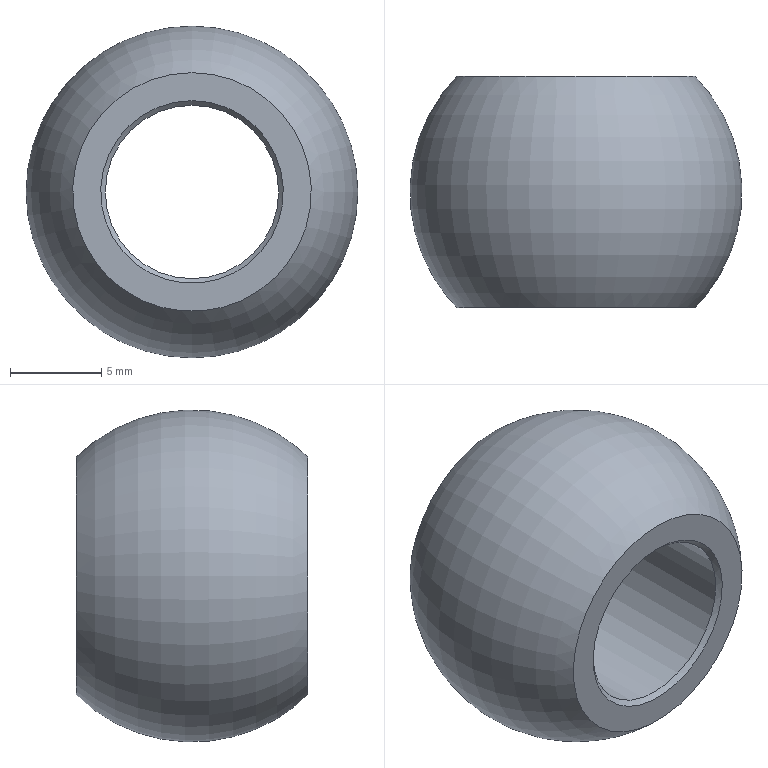Part | NX | features solid 2 | 1 solid | 6 faces | box 18.237 x 12.7 x 18.237 mm | volume 1876 mm3 | plane 2 | cone 2 | torus 1 | cylinder 1 | commonest cylinder face diameters 9.525 x1
STEP:
#1=CARTESIAN_POINT('',(0.,-6.35,5.016));
#2=VERTEX_POINT('',#1);
#3=CARTESIAN_POINT('',(0.,-6.35,0.));
#4=DIRECTION('',(0.,1.,0.));
#5=DIRECTION('',(0.,0.,1.));
#6=AXIS2_PLACEMENT_3D('',#3,#4,#5);
#7=CIRCLE('',#6,5.016);
#8=EDGE_CURVE('',#2,#2,#7,.T.);
#9=ORIENTED_EDGE('',*,*,#8,.T.);
#10=EDGE_LOOP('',(#9));
#11=FACE_BOUND('',#10,.T.);
#12=CARTESIAN_POINT('',(0.,-6.35,6.553));
#13=VERTEX_POINT('',#12);
#14=CARTESIAN_POINT('',(0.,-6.35,0.));
#15=DIRECTION('',(0.,1.,0.));
#16=DIRECTION('',(0.,0.,1.));
#17=AXIS2_PLACEMENT_3D('',#14,#15,#16);
#18=CIRCLE('',#17,6.553);
#19=EDGE_CURVE('',#13,#13,#18,.T.);
#20=ORIENTED_EDGE('',*,*,#19,.F.);
#21=EDGE_LOOP('',(#20));
#22=FACE_BOUND('',#21,.T.);
#23=CARTESIAN_POINT('',(0.,-6.35,4.763));
#24=DIRECTION('',(0.,1.,0.));
#25=DIRECTION('',(0.,0.,1.));
#26=AXIS2_PLACEMENT_3D('',#23,#24,#25);
#27=PLANE('',#26);
#28=ADVANCED_FACE('',(#11,#22),#27,.F.);
#29=CARTESIAN_POINT('',(0.,6.35,6.553));
#30=VERTEX_POINT('',#29);
#31=CARTESIAN_POINT('',(0.,6.35,0.));
#32=DIRECTION('',(0.,1.,0.));
#33=DIRECTION('',(0.,0.,1.));
#34=AXIS2_PLACEMENT_3D('',#31,#32,#33);
#35=CIRCLE('',#34,6.553);
#36=EDGE_CURVE('',#30,#30,#35,.T.);
#37=ORIENTED_EDGE('',*,*,#36,.F.);
#38=EDGE_LOOP('',(#37));
#39=FACE_BOUND('',#38,.T.);
#40=ORIENTED_EDGE('',*,*,#19,.T.);
#41=EDGE_LOOP('',(#40));
#42=FACE_BOUND('',#41,.T.);
#43=CARTESIAN_POINT('',(0.,0.,0.));
#44=DIRECTION('',(0.,1.,0.));
#45=DIRECTION('',(0.,0.,1.));
#46=AXIS2_PLACEMENT_3D('',#43,#44,#45);
#47=DEGENERATE_TOROIDAL_SURFACE('',#46,0.02301,9.142,.F.);
#48=ADVANCED_FACE('',(#39,#42),#47,.F.);
#49=CARTESIAN_POINT('',(0.,6.35,-5.016));
#50=VERTEX_POINT('',#49);
#51=CARTESIAN_POINT('',(0.,6.35,0.));
#52=DIRECTION('',(0.,-1.,0.));
#53=DIRECTION('',(0.,0.,-1.));
#54=AXIS2_PLACEMENT_3D('',#51,#52,#53);
#55=CIRCLE('',#54,5.016);
#56=EDGE_CURVE('',#50,#50,#55,.T.);
#57=ORIENTED_EDGE('',*,*,#56,.T.);
#58=EDGE_LOOP('',(#57));
#59=FACE_BOUND('',#58,.T.);
#60=ORIENTED_EDGE('',*,*,#36,.T.);
#61=EDGE_LOOP('',(#60));
#62=FACE_BOUND('',#61,.T.);
#63=CARTESIAN_POINT('',(0.,6.35,6.553));
#64=DIRECTION('',(0.,-1.,0.));
#65=DIRECTION('',(0.,0.,-1.));
#66=AXIS2_PLACEMENT_3D('',#63,#64,#65);
#67=PLANE('',#66);
#68=ADVANCED_FACE('',(#59,#62),#67,.F.);
#69=CARTESIAN_POINT('',(0.,-6.096,4.763));
#70=VERTEX_POINT('',#69);
#71=CARTESIAN_POINT('',(0.,-6.096,0.));
#72=DIRECTION('',(0.,1.,0.));
#73=DIRECTION('',(0.,0.,1.));
#74=AXIS2_PLACEMENT_3D('',#71,#72,#73);
#75=CIRCLE('',#74,4.763);
#76=EDGE_CURVE('',#70,#70,#75,.F.);
#77=ORIENTED_EDGE('',*,*,#76,.T.);
#78=EDGE_LOOP('',(#77));
#79=FACE_BOUND('',#78,.T.);
#80=CARTESIAN_POINT('',(0.,6.096,-4.763));
#81=VERTEX_POINT('',#80);
#82=CARTESIAN_POINT('',(0.,6.096,0.));
#83=DIRECTION('',(0.,-1.,0.));
#84=DIRECTION('',(0.,0.,-1.));
#85=AXIS2_PLACEMENT_3D('',#82,#83,#84);
#86=CIRCLE('',#85,4.763);
#87=EDGE_CURVE('',#81,#81,#86,.F.);
#88=ORIENTED_EDGE('',*,*,#87,.T.);
#89=EDGE_LOOP('',(#88));
#90=FACE_BOUND('',#89,.T.);
#91=CARTESIAN_POINT('',(0.,0.,0.));
#92=DIRECTION('',(0.,1.,0.));
#93=DIRECTION('',(0.,0.,1.));
#94=AXIS2_PLACEMENT_3D('',#91,#92,#93);
#95=CYLINDRICAL_SURFACE('',#94,4.763);
#96=ADVANCED_FACE('',(#79,#90),#95,.F.);
#97=ORIENTED_EDGE('',*,*,#76,.F.);
#98=EDGE_LOOP('',(#97));
#99=FACE_BOUND('',#98,.T.);
#100=ORIENTED_EDGE('',*,*,#8,.F.);
#101=EDGE_LOOP('',(#100));
#102=FACE_BOUND('',#101,.T.);
#103=CARTESIAN_POINT('',(0.,-6.35,0.));
#104=DIRECTION('',(0.,-1.,0.));
#105=DIRECTION('',(0.,0.,-1.));
#106=AXIS2_PLACEMENT_3D('',#103,#104,#105);
#107=CONICAL_SURFACE('',#106,5.016,0.7854);
#108=ADVANCED_FACE('',(#99,#102),#107,.F.);
#109=ORIENTED_EDGE('',*,*,#56,.F.);
#110=EDGE_LOOP('',(#109));
#111=FACE_BOUND('',#110,.T.);
#112=ORIENTED_EDGE('',*,*,#87,.F.);
#113=EDGE_LOOP('',(#112));
#114=FACE_BOUND('',#113,.T.);
#115=CARTESIAN_POINT('',(0.,6.096,0.));
#116=DIRECTION('',(0.,1.,0.));
#117=DIRECTION('',(0.,0.,1.));
#118=AXIS2_PLACEMENT_3D('',#115,#116,#117);
#119=CONICAL_SURFACE('',#118,4.763,0.7854);
#120=ADVANCED_FACE('',(#111,#114),#119,.F.);
#121=CLOSED_SHELL('',(#28,#48,#68,#96,#108,#120));
#122=MANIFOLD_SOLID_BREP('',#121);
#123=(LENGTH_UNIT()NAMED_UNIT(*)SI_UNIT(.MILLI.,.METRE.));
#124=UNCERTAINTY_MEASURE_WITH_UNIT(LENGTH_MEASURE(0.00001),#123,'','');
#125=(NAMED_UNIT(*)PLANE_ANGLE_UNIT()SI_UNIT($,.RADIAN.));
#126=(NAMED_UNIT(*)SI_UNIT($,.STERADIAN.)SOLID_ANGLE_UNIT());
#127=(GEOMETRIC_REPRESENTATION_CONTEXT(3)GLOBAL_UNCERTAINTY_ASSIGNED_CONTEXT((#124))GLOBAL_UNIT_ASSIGNED_CONTEXT((#123,#125,#126))REPRESENTATION_CONTEXT('',''));
#128=ADVANCED_BREP_SHAPE_REPRESENTATION('',(#122),#127);